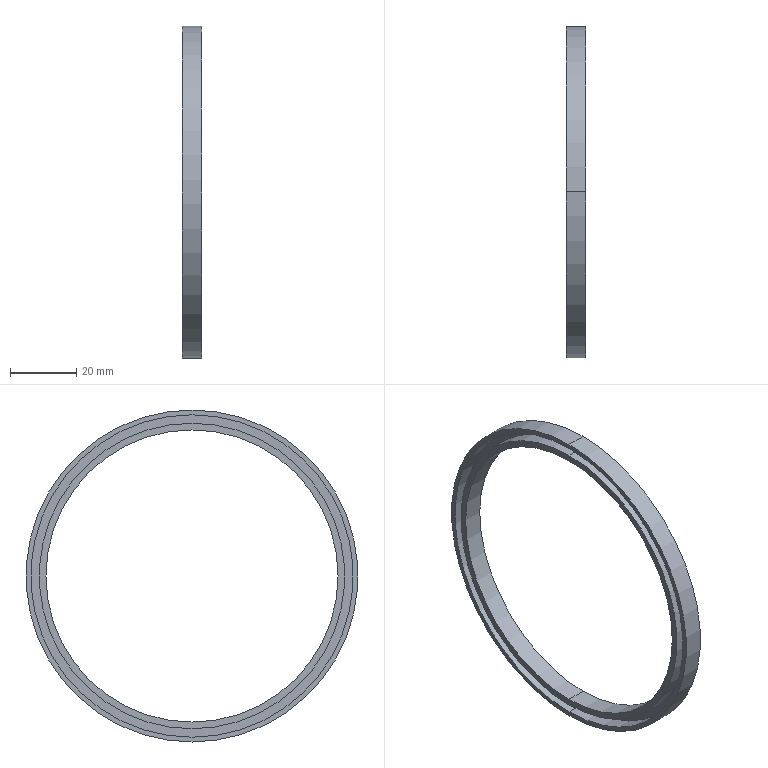Part | SolidWorks | features Revolution 1 | 1 solid | 12 faces | box 6 x 100 x 100 mm | volume 7223 mm3 | cylinder 8 | plane 4 | commonest cylinder face diameters 88 x2 92 x2 97.1 x2 100 x2
STEP:
#1=CARTESIAN_POINT('',(-50.,0.,48.55));
#2=VERTEX_POINT('',#1);
#3=CARTESIAN_POINT('',(-50.,0.,-48.55));
#4=VERTEX_POINT('',#3);
#5=CARTESIAN_POINT('',(-50.,0.,0.));
#6=DIRECTION('',(1.,0.,0.));
#7=DIRECTION('',(0.,0.,-1.));
#8=AXIS2_PLACEMENT_3D('',#5,#6,#7);
#9=CIRCLE('',#8,48.55);
#10=EDGE_CURVE('',#2,#4,#9,.T.);
#11=ORIENTED_EDGE('',*,*,#10,.F.);
#12=CARTESIAN_POINT('',(-45.5,0.,48.55));
#13=VERTEX_POINT('',#12);
#14=CARTESIAN_POINT('',(0.,0.,48.55));
#15=DIRECTION('',(1.,0.,0.));
#16=VECTOR('',#15,1000.);
#17=LINE('',#14,#16);
#18=EDGE_CURVE('',#2,#13,#17,.T.);
#19=ORIENTED_EDGE('',*,*,#18,.T.);
#20=CARTESIAN_POINT('',(-45.5,0.,-48.55));
#21=VERTEX_POINT('',#20);
#22=CARTESIAN_POINT('',(-45.5,0.,0.));
#23=DIRECTION('',(1.,0.,0.));
#24=DIRECTION('',(0.,0.,-1.));
#25=AXIS2_PLACEMENT_3D('',#22,#23,#24);
#26=CIRCLE('',#25,48.55);
#27=EDGE_CURVE('',#13,#21,#26,.T.);
#28=ORIENTED_EDGE('',*,*,#27,.T.);
#29=CARTESIAN_POINT('',(0.,0.,-48.55));
#30=DIRECTION('',(1.,0.,0.));
#31=VECTOR('',#30,1000.);
#32=LINE('',#29,#31);
#33=EDGE_CURVE('',#4,#21,#32,.T.);
#34=ORIENTED_EDGE('',*,*,#33,.F.);
#35=EDGE_LOOP('',(#11,#19,#28,#34));
#36=FACE_OUTER_BOUND('',#35,.T.);
#37=CARTESIAN_POINT('',(0.,0.,0.));
#38=DIRECTION('',(1.,0.,0.));
#39=DIRECTION('',(0.,0.,-1.));
#40=AXIS2_PLACEMENT_3D('',#37,#38,#39);
#41=CYLINDRICAL_SURFACE('',#40,48.55);
#42=ADVANCED_FACE('',(#36),#41,.F.);
#43=CARTESIAN_POINT('',(-50.,0.,-46.));
#44=VERTEX_POINT('',#43);
#45=CARTESIAN_POINT('',(-50.,0.,46.));
#46=VERTEX_POINT('',#45);
#47=CARTESIAN_POINT('',(-50.,0.,0.));
#48=DIRECTION('',(1.,0.,0.));
#49=DIRECTION('',(0.,0.,-1.));
#50=AXIS2_PLACEMENT_3D('',#47,#48,#49);
#51=CIRCLE('',#50,46.);
#52=EDGE_CURVE('',#44,#46,#51,.T.);
#53=ORIENTED_EDGE('',*,*,#52,.T.);
#54=CARTESIAN_POINT('',(-45.5,0.,46.));
#55=VERTEX_POINT('',#54);
#56=CARTESIAN_POINT('',(0.,0.,46.));
#57=DIRECTION('',(1.,0.,0.));
#58=VECTOR('',#57,1000.);
#59=LINE('',#56,#58);
#60=EDGE_CURVE('',#46,#55,#59,.T.);
#61=ORIENTED_EDGE('',*,*,#60,.T.);
#62=CARTESIAN_POINT('',(-45.5,0.,-46.));
#63=VERTEX_POINT('',#62);
#64=CARTESIAN_POINT('',(-45.5,0.,0.));
#65=DIRECTION('',(1.,0.,0.));
#66=DIRECTION('',(0.,0.,-1.));
#67=AXIS2_PLACEMENT_3D('',#64,#65,#66);
#68=CIRCLE('',#67,46.);
#69=EDGE_CURVE('',#63,#55,#68,.T.);
#70=ORIENTED_EDGE('',*,*,#69,.F.);
#71=CARTESIAN_POINT('',(0.,0.,-46.));
#72=DIRECTION('',(1.,0.,0.));
#73=VECTOR('',#72,1000.);
#74=LINE('',#71,#73);
#75=EDGE_CURVE('',#44,#63,#74,.T.);
#76=ORIENTED_EDGE('',*,*,#75,.F.);
#77=EDGE_LOOP('',(#53,#61,#70,#76));
#78=FACE_OUTER_BOUND('',#77,.T.);
#79=CARTESIAN_POINT('',(0.,0.,0.));
#80=DIRECTION('',(1.,0.,0.));
#81=DIRECTION('',(0.,0.,-1.));
#82=AXIS2_PLACEMENT_3D('',#79,#80,#81);
#83=CYLINDRICAL_SURFACE('',#82,46.);
#84=ADVANCED_FACE('',(#78),#83,.T.);
#85=CARTESIAN_POINT('',(-50.,0.,44.));
#86=VERTEX_POINT('',#85);
#87=CARTESIAN_POINT('',(-50.,0.,-44.));
#88=VERTEX_POINT('',#87);
#89=CARTESIAN_POINT('',(-50.,0.,0.));
#90=DIRECTION('',(1.,0.,0.));
#91=DIRECTION('',(0.,0.,-1.));
#92=AXIS2_PLACEMENT_3D('',#89,#90,#91);
#93=CIRCLE('',#92,44.);
#94=EDGE_CURVE('',#86,#88,#93,.T.);
#95=ORIENTED_EDGE('',*,*,#94,.F.);
#96=CARTESIAN_POINT('',(-44.,0.,44.));
#97=VERTEX_POINT('',#96);
#98=CARTESIAN_POINT('',(0.,0.,44.));
#99=DIRECTION('',(1.,0.,0.));
#100=VECTOR('',#99,1000.);
#101=LINE('',#98,#100);
#102=EDGE_CURVE('',#86,#97,#101,.T.);
#103=ORIENTED_EDGE('',*,*,#102,.T.);
#104=CARTESIAN_POINT('',(-44.,0.,-44.));
#105=VERTEX_POINT('',#104);
#106=CARTESIAN_POINT('',(-44.,0.,0.));
#107=DIRECTION('',(1.,0.,0.));
#108=DIRECTION('',(0.,0.,-1.));
#109=AXIS2_PLACEMENT_3D('',#106,#107,#108);
#110=CIRCLE('',#109,44.);
#111=EDGE_CURVE('',#97,#105,#110,.T.);
#112=ORIENTED_EDGE('',*,*,#111,.T.);
#113=CARTESIAN_POINT('',(0.,0.,-44.));
#114=DIRECTION('',(1.,0.,0.));
#115=VECTOR('',#114,1000.);
#116=LINE('',#113,#115);
#117=EDGE_CURVE('',#88,#105,#116,.T.);
#118=ORIENTED_EDGE('',*,*,#117,.F.);
#119=EDGE_LOOP('',(#95,#103,#112,#118));
#120=FACE_OUTER_BOUND('',#119,.T.);
#121=CARTESIAN_POINT('',(0.,0.,0.));
#122=DIRECTION('',(1.,0.,0.));
#123=DIRECTION('',(0.,0.,-1.));
#124=AXIS2_PLACEMENT_3D('',#121,#122,#123);
#125=CYLINDRICAL_SURFACE('',#124,44.);
#126=ADVANCED_FACE('',(#120),#125,.F.);
#127=CARTESIAN_POINT('',(-50.,0.,-50.));
#128=VERTEX_POINT('',#127);
#129=CARTESIAN_POINT('',(-50.,0.,50.));
#130=VERTEX_POINT('',#129);
#131=CARTESIAN_POINT('',(-50.,0.,0.));
#132=DIRECTION('',(1.,0.,0.));
#133=DIRECTION('',(0.,0.,-1.));
#134=AXIS2_PLACEMENT_3D('',#131,#132,#133);
#135=CIRCLE('',#134,50.);
#136=EDGE_CURVE('',#128,#130,#135,.T.);
#137=ORIENTED_EDGE('',*,*,#136,.T.);
#138=CARTESIAN_POINT('',(-44.,0.,50.));
#139=VERTEX_POINT('',#138);
#140=CARTESIAN_POINT('',(0.,0.,50.));
#141=DIRECTION('',(1.,0.,0.));
#142=VECTOR('',#141,1000.);
#143=LINE('',#140,#142);
#144=EDGE_CURVE('',#130,#139,#143,.T.);
#145=ORIENTED_EDGE('',*,*,#144,.T.);
#146=CARTESIAN_POINT('',(-44.,0.,-50.));
#147=VERTEX_POINT('',#146);
#148=CARTESIAN_POINT('',(-44.,0.,0.));
#149=DIRECTION('',(1.,0.,0.));
#150=DIRECTION('',(0.,0.,-1.));
#151=AXIS2_PLACEMENT_3D('',#148,#149,#150);
#152=CIRCLE('',#151,50.);
#153=EDGE_CURVE('',#147,#139,#152,.T.);
#154=ORIENTED_EDGE('',*,*,#153,.F.);
#155=CARTESIAN_POINT('',(0.,0.,-50.));
#156=DIRECTION('',(1.,0.,0.));
#157=VECTOR('',#156,1000.);
#158=LINE('',#155,#157);
#159=EDGE_CURVE('',#128,#147,#158,.T.);
#160=ORIENTED_EDGE('',*,*,#159,.F.);
#161=EDGE_LOOP('',(#137,#145,#154,#160));
#162=FACE_OUTER_BOUND('',#161,.T.);
#163=CARTESIAN_POINT('',(0.,0.,0.));
#164=DIRECTION('',(1.,0.,0.));
#165=DIRECTION('',(0.,0.,-1.));
#166=AXIS2_PLACEMENT_3D('',#163,#164,#165);
#167=CYLINDRICAL_SURFACE('',#166,50.);
#168=ADVANCED_FACE('',(#162),#167,.T.);
#169=ORIENTED_EDGE('',*,*,#136,.F.);
#170=CARTESIAN_POINT('',(-50.,0.,0.));
#171=DIRECTION('',(1.,0.,0.));
#172=DIRECTION('',(0.,0.,-1.));
#173=AXIS2_PLACEMENT_3D('',#170,#171,#172);
#174=CIRCLE('',#173,50.);
#175=EDGE_CURVE('',#130,#128,#174,.T.);
#176=ORIENTED_EDGE('',*,*,#175,.F.);
#177=EDGE_LOOP('',(#169,#176));
#178=FACE_OUTER_BOUND('',#177,.T.);
#179=CARTESIAN_POINT('',(-50.,0.,0.));
#180=DIRECTION('',(1.,0.,0.));
#181=DIRECTION('',(0.,0.,-1.));
#182=AXIS2_PLACEMENT_3D('',#179,#180,#181);
#183=CIRCLE('',#182,48.55);
#184=EDGE_CURVE('',#4,#2,#183,.T.);
#185=ORIENTED_EDGE('',*,*,#184,.T.);
#186=ORIENTED_EDGE('',*,*,#10,.T.);
#187=EDGE_LOOP('',(#185,#186));
#188=FACE_BOUND('',#187,.T.);
#189=CARTESIAN_POINT('',(-50.,48.55,0.));
#190=DIRECTION('',(1.,0.,0.));
#191=DIRECTION('',(0.,0.,-1.));
#192=AXIS2_PLACEMENT_3D('',#189,#190,#191);
#193=PLANE('',#192);
#194=ADVANCED_FACE('',(#178,#188),#193,.F.);
#195=ORIENTED_EDGE('',*,*,#144,.F.);
#196=ORIENTED_EDGE('',*,*,#175,.T.);
#197=ORIENTED_EDGE('',*,*,#159,.T.);
#198=CARTESIAN_POINT('',(-44.,0.,0.));
#199=DIRECTION('',(1.,0.,0.));
#200=DIRECTION('',(0.,0.,-1.));
#201=AXIS2_PLACEMENT_3D('',#198,#199,#200);
#202=CIRCLE('',#201,50.);
#203=EDGE_CURVE('',#139,#147,#202,.T.);
#204=ORIENTED_EDGE('',*,*,#203,.F.);
#205=EDGE_LOOP('',(#195,#196,#197,#204));
#206=FACE_OUTER_BOUND('',#205,.T.);
#207=CARTESIAN_POINT('',(0.,0.,0.));
#208=DIRECTION('',(1.,0.,0.));
#209=DIRECTION('',(0.,0.,-1.));
#210=AXIS2_PLACEMENT_3D('',#207,#208,#209);
#211=CYLINDRICAL_SURFACE('',#210,50.);
#212=ADVANCED_FACE('',(#206),#211,.T.);
#213=CARTESIAN_POINT('',(-44.,0.,0.));
#214=DIRECTION('',(1.,0.,0.));
#215=DIRECTION('',(0.,0.,-1.));
#216=AXIS2_PLACEMENT_3D('',#213,#214,#215);
#217=CIRCLE('',#216,44.);
#218=EDGE_CURVE('',#105,#97,#217,.T.);
#219=ORIENTED_EDGE('',*,*,#218,.F.);
#220=ORIENTED_EDGE('',*,*,#111,.F.);
#221=EDGE_LOOP('',(#219,#220));
#222=FACE_BOUND('',#221,.T.);
#223=ORIENTED_EDGE('',*,*,#153,.T.);
#224=ORIENTED_EDGE('',*,*,#203,.T.);
#225=EDGE_LOOP('',(#223,#224));
#226=FACE_OUTER_BOUND('',#225,.T.);
#227=CARTESIAN_POINT('',(-44.,50.,0.));
#228=DIRECTION('',(-1.,0.,0.));
#229=DIRECTION('',(0.,0.,1.));
#230=AXIS2_PLACEMENT_3D('',#227,#228,#229);
#231=PLANE('',#230);
#232=ADVANCED_FACE('',(#222,#226),#231,.F.);
#233=ORIENTED_EDGE('',*,*,#102,.F.);
#234=CARTESIAN_POINT('',(-50.,0.,0.));
#235=DIRECTION('',(1.,0.,0.));
#236=DIRECTION('',(0.,0.,-1.));
#237=AXIS2_PLACEMENT_3D('',#234,#235,#236);
#238=CIRCLE('',#237,44.);
#239=EDGE_CURVE('',#88,#86,#238,.T.);
#240=ORIENTED_EDGE('',*,*,#239,.F.);
#241=ORIENTED_EDGE('',*,*,#117,.T.);
#242=ORIENTED_EDGE('',*,*,#218,.T.);
#243=EDGE_LOOP('',(#233,#240,#241,#242));
#244=FACE_OUTER_BOUND('',#243,.T.);
#245=CARTESIAN_POINT('',(0.,0.,0.));
#246=DIRECTION('',(1.,0.,0.));
#247=DIRECTION('',(0.,0.,-1.));
#248=AXIS2_PLACEMENT_3D('',#245,#246,#247);
#249=CYLINDRICAL_SURFACE('',#248,44.);
#250=ADVANCED_FACE('',(#244),#249,.F.);
#251=ORIENTED_EDGE('',*,*,#52,.F.);
#252=CARTESIAN_POINT('',(-50.,0.,0.));
#253=DIRECTION('',(1.,0.,0.));
#254=DIRECTION('',(0.,0.,-1.));
#255=AXIS2_PLACEMENT_3D('',#252,#253,#254);
#256=CIRCLE('',#255,46.);
#257=EDGE_CURVE('',#46,#44,#256,.T.);
#258=ORIENTED_EDGE('',*,*,#257,.F.);
#259=EDGE_LOOP('',(#251,#258));
#260=FACE_OUTER_BOUND('',#259,.T.);
#261=ORIENTED_EDGE('',*,*,#239,.T.);
#262=ORIENTED_EDGE('',*,*,#94,.T.);
#263=EDGE_LOOP('',(#261,#262));
#264=FACE_BOUND('',#263,.T.);
#265=CARTESIAN_POINT('',(-50.,44.,0.));
#266=DIRECTION('',(1.,0.,0.));
#267=DIRECTION('',(0.,0.,-1.));
#268=AXIS2_PLACEMENT_3D('',#265,#266,#267);
#269=PLANE('',#268);
#270=ADVANCED_FACE('',(#260,#264),#269,.F.);
#271=ORIENTED_EDGE('',*,*,#60,.F.);
#272=ORIENTED_EDGE('',*,*,#257,.T.);
#273=ORIENTED_EDGE('',*,*,#75,.T.);
#274=CARTESIAN_POINT('',(-45.5,0.,0.));
#275=DIRECTION('',(1.,0.,0.));
#276=DIRECTION('',(0.,0.,-1.));
#277=AXIS2_PLACEMENT_3D('',#274,#275,#276);
#278=CIRCLE('',#277,46.);
#279=EDGE_CURVE('',#55,#63,#278,.T.);
#280=ORIENTED_EDGE('',*,*,#279,.F.);
#281=EDGE_LOOP('',(#271,#272,#273,#280));
#282=FACE_OUTER_BOUND('',#281,.T.);
#283=CARTESIAN_POINT('',(0.,0.,0.));
#284=DIRECTION('',(1.,0.,0.));
#285=DIRECTION('',(0.,0.,-1.));
#286=AXIS2_PLACEMENT_3D('',#283,#284,#285);
#287=CYLINDRICAL_SURFACE('',#286,46.);
#288=ADVANCED_FACE('',(#282),#287,.T.);
#289=CARTESIAN_POINT('',(-45.5,0.,0.));
#290=DIRECTION('',(1.,0.,0.));
#291=DIRECTION('',(0.,0.,-1.));
#292=AXIS2_PLACEMENT_3D('',#289,#290,#291);
#293=CIRCLE('',#292,48.55);
#294=EDGE_CURVE('',#21,#13,#293,.T.);
#295=ORIENTED_EDGE('',*,*,#294,.F.);
#296=ORIENTED_EDGE('',*,*,#27,.F.);
#297=EDGE_LOOP('',(#295,#296));
#298=FACE_OUTER_BOUND('',#297,.T.);
#299=ORIENTED_EDGE('',*,*,#69,.T.);
#300=ORIENTED_EDGE('',*,*,#279,.T.);
#301=EDGE_LOOP('',(#299,#300));
#302=FACE_BOUND('',#301,.T.);
#303=CARTESIAN_POINT('',(-45.5,46.,0.));
#304=DIRECTION('',(1.,0.,0.));
#305=DIRECTION('',(0.,0.,-1.));
#306=AXIS2_PLACEMENT_3D('',#303,#304,#305);
#307=PLANE('',#306);
#308=ADVANCED_FACE('',(#298,#302),#307,.F.);
#309=ORIENTED_EDGE('',*,*,#18,.F.);
#310=ORIENTED_EDGE('',*,*,#184,.F.);
#311=ORIENTED_EDGE('',*,*,#33,.T.);
#312=ORIENTED_EDGE('',*,*,#294,.T.);
#313=EDGE_LOOP('',(#309,#310,#311,#312));
#314=FACE_OUTER_BOUND('',#313,.T.);
#315=CARTESIAN_POINT('',(0.,0.,0.));
#316=DIRECTION('',(1.,0.,0.));
#317=DIRECTION('',(0.,0.,-1.));
#318=AXIS2_PLACEMENT_3D('',#315,#316,#317);
#319=CYLINDRICAL_SURFACE('',#318,48.55);
#320=ADVANCED_FACE('',(#314),#319,.F.);
#321=CLOSED_SHELL('',(#42,#84,#126,#168,#194,#212,#232,#250,#270,#288,#308,#320));
#322=MANIFOLD_SOLID_BREP('',#321);
#323=CARTESIAN_POINT('',(0.,0.,0.));
#324=DIRECTION('',(0.,0.,1.));
#325=DIRECTION('',(1.,0.,0.));
#326=AXIS2_PLACEMENT_3D('',#323,#324,#325);
#327=(LENGTH_UNIT()NAMED_UNIT(*)SI_UNIT(.MILLI.,.METRE.));
#328=UNCERTAINTY_MEASURE_WITH_UNIT(LENGTH_MEASURE(0.00001),#327,'','');
#329=(NAMED_UNIT(*)PLANE_ANGLE_UNIT()SI_UNIT($,.RADIAN.));
#330=(NAMED_UNIT(*)SI_UNIT($,.STERADIAN.)SOLID_ANGLE_UNIT());
#331=(GEOMETRIC_REPRESENTATION_CONTEXT(3)GLOBAL_UNCERTAINTY_ASSIGNED_CONTEXT((#328))GLOBAL_UNIT_ASSIGNED_CONTEXT((#327,#329,#330))REPRESENTATION_CONTEXT('',''));
#332=ADVANCED_BREP_SHAPE_REPRESENTATION('',(#322,#326),#331);